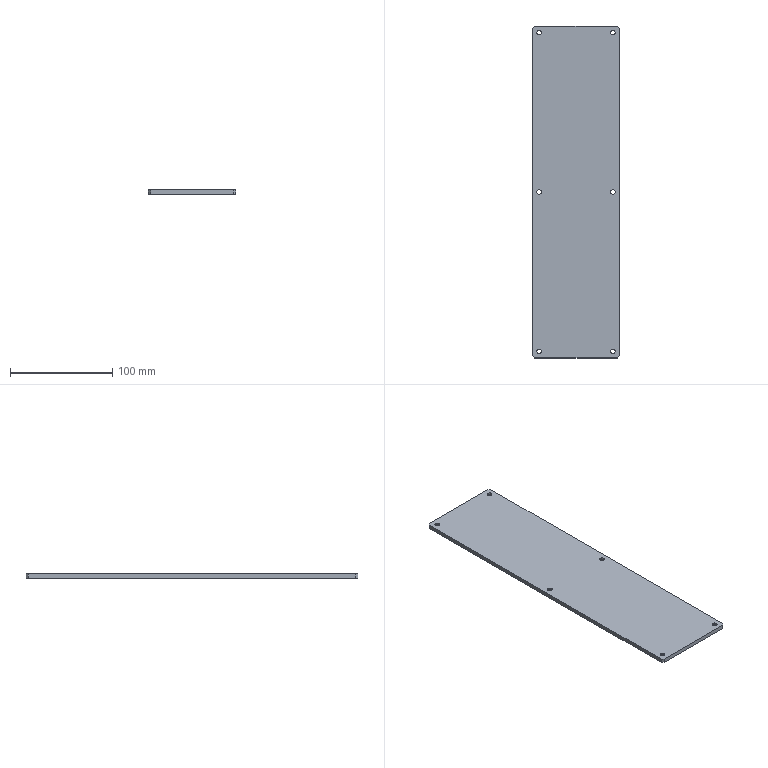Part | STEP file | 11-FG-SZ02911 | 1 solid | 34 faces | box 85 x 324 x 4 mm | volume 109466 mm3 | cone 12 | cylinder 12 | plane 10 | commonest cylinder face diameters 4.5 x12
STEP:
#1=CARTESIAN_POINT('',(-33.75,-155.5,2.23));
#2=VERTEX_POINT('',#1);
#3=CARTESIAN_POINT('',(-38.25,-155.5,2.23));
#4=VERTEX_POINT('',#3);
#5=CARTESIAN_POINT('',(-36.,-155.5,2.23));
#6=DIRECTION('',(0.,0.,-1.));
#7=DIRECTION('',(-1.,0.,0.));
#8=AXIS2_PLACEMENT_3D('',#5,#6,#7);
#9=CIRCLE('',#8,2.25);
#10=EDGE_CURVE('',#2,#4,#9,.T.);
#11=ORIENTED_EDGE('',*,*,#10,.F.);
#12=CARTESIAN_POINT('',(-31.52,-155.5,0.));
#13=VERTEX_POINT('',#12);
#14=CARTESIAN_POINT('',(-31.52,-155.5,0.));
#15=DIRECTION('',(0.7071,0.,-0.7071));
#16=VECTOR('',#15,1000.);
#17=LINE('',#14,#16);
#18=EDGE_CURVE('',#2,#13,#17,.T.);
#19=ORIENTED_EDGE('',*,*,#18,.T.);
#20=CARTESIAN_POINT('',(-40.48,-155.5,0.));
#21=VERTEX_POINT('',#20);
#22=CARTESIAN_POINT('',(-36.,-155.5,0.));
#23=DIRECTION('',(0.,0.,-1.));
#24=DIRECTION('',(-1.,0.,0.));
#25=AXIS2_PLACEMENT_3D('',#22,#23,#24);
#26=CIRCLE('',#25,4.48);
#27=EDGE_CURVE('',#13,#21,#26,.T.);
#28=ORIENTED_EDGE('',*,*,#27,.T.);
#29=CARTESIAN_POINT('',(-40.48,-155.5,0.));
#30=DIRECTION('',(-0.7071,0.,-0.7071));
#31=VECTOR('',#30,1000.);
#32=LINE('',#29,#31);
#33=EDGE_CURVE('',#4,#21,#32,.T.);
#34=ORIENTED_EDGE('',*,*,#33,.F.);
#35=EDGE_LOOP('',(#11,#19,#28,#34));
#36=FACE_OUTER_BOUND('',#35,.T.);
#37=CARTESIAN_POINT('',(-36.,-155.5,0.));
#38=DIRECTION('',(0.,0.,-1.));
#39=DIRECTION('',(-1.,0.,0.));
#40=AXIS2_PLACEMENT_3D('',#37,#38,#39);
#41=CONICAL_SURFACE('',#40,4.48,0.7854);
#42=ADVANCED_FACE('',(#36),#41,.F.);
#43=CARTESIAN_POINT('',(-38.25,-155.5,4.));
#44=VERTEX_POINT('',#43);
#45=CARTESIAN_POINT('',(-33.75,-155.5,4.));
#46=VERTEX_POINT('',#45);
#47=CARTESIAN_POINT('',(-36.,-155.5,4.));
#48=DIRECTION('',(0.,0.,1.));
#49=DIRECTION('',(1.,0.,0.));
#50=AXIS2_PLACEMENT_3D('',#47,#48,#49);
#51=CIRCLE('',#50,2.25);
#52=EDGE_CURVE('',#44,#46,#51,.T.);
#53=ORIENTED_EDGE('',*,*,#52,.T.);
#54=CARTESIAN_POINT('',(-33.75,-155.5,0.));
#55=DIRECTION('',(0.,0.,-1.));
#56=VECTOR('',#55,1000.);
#57=LINE('',#54,#56);
#58=EDGE_CURVE('',#46,#2,#57,.T.);
#59=ORIENTED_EDGE('',*,*,#58,.T.);
#60=ORIENTED_EDGE('',*,*,#10,.T.);
#61=CARTESIAN_POINT('',(-38.25,-155.5,0.));
#62=DIRECTION('',(0.,0.,-1.));
#63=VECTOR('',#62,1000.);
#64=LINE('',#61,#63);
#65=EDGE_CURVE('',#44,#4,#64,.T.);
#66=ORIENTED_EDGE('',*,*,#65,.F.);
#67=EDGE_LOOP('',(#53,#59,#60,#66));
#68=FACE_OUTER_BOUND('',#67,.T.);
#69=CARTESIAN_POINT('',(-36.,-155.5,0.));
#70=DIRECTION('',(0.,0.,-1.));
#71=DIRECTION('',(-1.,0.,0.));
#72=AXIS2_PLACEMENT_3D('',#69,#70,#71);
#73=CYLINDRICAL_SURFACE('',#72,2.25);
#74=ADVANCED_FACE('',(#68),#73,.F.);
#75=CARTESIAN_POINT('',(-33.75,155.5,2.23));
#76=VERTEX_POINT('',#75);
#77=CARTESIAN_POINT('',(-38.25,155.5,2.23));
#78=VERTEX_POINT('',#77);
#79=CARTESIAN_POINT('',(-36.,155.5,2.23));
#80=DIRECTION('',(0.,0.,-1.));
#81=DIRECTION('',(-1.,0.,0.));
#82=AXIS2_PLACEMENT_3D('',#79,#80,#81);
#83=CIRCLE('',#82,2.25);
#84=EDGE_CURVE('',#76,#78,#83,.T.);
#85=ORIENTED_EDGE('',*,*,#84,.F.);
#86=CARTESIAN_POINT('',(-31.52,155.5,0.));
#87=VERTEX_POINT('',#86);
#88=CARTESIAN_POINT('',(-31.52,155.5,0.));
#89=DIRECTION('',(0.7071,0.,-0.7071));
#90=VECTOR('',#89,1000.);
#91=LINE('',#88,#90);
#92=EDGE_CURVE('',#76,#87,#91,.T.);
#93=ORIENTED_EDGE('',*,*,#92,.T.);
#94=CARTESIAN_POINT('',(-40.48,155.5,0.));
#95=VERTEX_POINT('',#94);
#96=CARTESIAN_POINT('',(-36.,155.5,0.));
#97=DIRECTION('',(0.,0.,-1.));
#98=DIRECTION('',(-1.,0.,0.));
#99=AXIS2_PLACEMENT_3D('',#96,#97,#98);
#100=CIRCLE('',#99,4.48);
#101=EDGE_CURVE('',#87,#95,#100,.T.);
#102=ORIENTED_EDGE('',*,*,#101,.T.);
#103=CARTESIAN_POINT('',(-40.48,155.5,0.));
#104=DIRECTION('',(-0.7071,0.,-0.7071));
#105=VECTOR('',#104,1000.);
#106=LINE('',#103,#105);
#107=EDGE_CURVE('',#78,#95,#106,.T.);
#108=ORIENTED_EDGE('',*,*,#107,.F.);
#109=EDGE_LOOP('',(#85,#93,#102,#108));
#110=FACE_OUTER_BOUND('',#109,.T.);
#111=CARTESIAN_POINT('',(-36.,155.5,0.));
#112=DIRECTION('',(0.,0.,-1.));
#113=DIRECTION('',(-1.,0.,0.));
#114=AXIS2_PLACEMENT_3D('',#111,#112,#113);
#115=CONICAL_SURFACE('',#114,4.48,0.7854);
#116=ADVANCED_FACE('',(#110),#115,.F.);
#117=CARTESIAN_POINT('',(-38.25,155.5,4.));
#118=VERTEX_POINT('',#117);
#119=CARTESIAN_POINT('',(-33.75,155.5,4.));
#120=VERTEX_POINT('',#119);
#121=CARTESIAN_POINT('',(-36.,155.5,4.));
#122=DIRECTION('',(0.,0.,1.));
#123=DIRECTION('',(1.,0.,0.));
#124=AXIS2_PLACEMENT_3D('',#121,#122,#123);
#125=CIRCLE('',#124,2.25);
#126=EDGE_CURVE('',#118,#120,#125,.T.);
#127=ORIENTED_EDGE('',*,*,#126,.T.);
#128=CARTESIAN_POINT('',(-33.75,155.5,0.));
#129=DIRECTION('',(0.,0.,-1.));
#130=VECTOR('',#129,1000.);
#131=LINE('',#128,#130);
#132=EDGE_CURVE('',#120,#76,#131,.T.);
#133=ORIENTED_EDGE('',*,*,#132,.T.);
#134=ORIENTED_EDGE('',*,*,#84,.T.);
#135=CARTESIAN_POINT('',(-38.25,155.5,0.));
#136=DIRECTION('',(0.,0.,-1.));
#137=VECTOR('',#136,1000.);
#138=LINE('',#135,#137);
#139=EDGE_CURVE('',#118,#78,#138,.T.);
#140=ORIENTED_EDGE('',*,*,#139,.F.);
#141=EDGE_LOOP('',(#127,#133,#134,#140));
#142=FACE_OUTER_BOUND('',#141,.T.);
#143=CARTESIAN_POINT('',(-36.,155.5,0.));
#144=DIRECTION('',(0.,0.,-1.));
#145=DIRECTION('',(-1.,0.,0.));
#146=AXIS2_PLACEMENT_3D('',#143,#144,#145);
#147=CYLINDRICAL_SURFACE('',#146,2.25);
#148=ADVANCED_FACE('',(#142),#147,.F.);
#149=CARTESIAN_POINT('',(-33.75,0.,2.23));
#150=VERTEX_POINT('',#149);
#151=CARTESIAN_POINT('',(-38.25,0.,2.23));
#152=VERTEX_POINT('',#151);
#153=CARTESIAN_POINT('',(-36.,0.,2.23));
#154=DIRECTION('',(0.,0.,-1.));
#155=DIRECTION('',(-1.,0.,0.));
#156=AXIS2_PLACEMENT_3D('',#153,#154,#155);
#157=CIRCLE('',#156,2.25);
#158=EDGE_CURVE('',#150,#152,#157,.T.);
#159=ORIENTED_EDGE('',*,*,#158,.F.);
#160=CARTESIAN_POINT('',(-31.52,0.,0.));
#161=VERTEX_POINT('',#160);
#162=CARTESIAN_POINT('',(-31.52,0.,0.));
#163=DIRECTION('',(0.7071,0.,-0.7071));
#164=VECTOR('',#163,1000.);
#165=LINE('',#162,#164);
#166=EDGE_CURVE('',#150,#161,#165,.T.);
#167=ORIENTED_EDGE('',*,*,#166,.T.);
#168=CARTESIAN_POINT('',(-40.48,0.,0.));
#169=VERTEX_POINT('',#168);
#170=CARTESIAN_POINT('',(-36.,0.,0.));
#171=DIRECTION('',(0.,0.,-1.));
#172=DIRECTION('',(-1.,0.,0.));
#173=AXIS2_PLACEMENT_3D('',#170,#171,#172);
#174=CIRCLE('',#173,4.48);
#175=EDGE_CURVE('',#161,#169,#174,.T.);
#176=ORIENTED_EDGE('',*,*,#175,.T.);
#177=CARTESIAN_POINT('',(-40.48,0.,0.));
#178=DIRECTION('',(-0.7071,0.,-0.7071));
#179=VECTOR('',#178,1000.);
#180=LINE('',#177,#179);
#181=EDGE_CURVE('',#152,#169,#180,.T.);
#182=ORIENTED_EDGE('',*,*,#181,.F.);
#183=EDGE_LOOP('',(#159,#167,#176,#182));
#184=FACE_OUTER_BOUND('',#183,.T.);
#185=CARTESIAN_POINT('',(-36.,0.,0.));
#186=DIRECTION('',(0.,0.,-1.));
#187=DIRECTION('',(-1.,0.,0.));
#188=AXIS2_PLACEMENT_3D('',#185,#186,#187);
#189=CONICAL_SURFACE('',#188,4.48,0.7854);
#190=ADVANCED_FACE('',(#184),#189,.F.);
#191=CARTESIAN_POINT('',(-38.25,0.,4.));
#192=VERTEX_POINT('',#191);
#193=CARTESIAN_POINT('',(-33.75,0.,4.));
#194=VERTEX_POINT('',#193);
#195=CARTESIAN_POINT('',(-36.,0.,4.));
#196=DIRECTION('',(0.,0.,1.));
#197=DIRECTION('',(1.,0.,0.));
#198=AXIS2_PLACEMENT_3D('',#195,#196,#197);
#199=CIRCLE('',#198,2.25);
#200=EDGE_CURVE('',#192,#194,#199,.T.);
#201=ORIENTED_EDGE('',*,*,#200,.T.);
#202=CARTESIAN_POINT('',(-33.75,0.,0.));
#203=DIRECTION('',(0.,0.,-1.));
#204=VECTOR('',#203,1000.);
#205=LINE('',#202,#204);
#206=EDGE_CURVE('',#194,#150,#205,.T.);
#207=ORIENTED_EDGE('',*,*,#206,.T.);
#208=ORIENTED_EDGE('',*,*,#158,.T.);
#209=CARTESIAN_POINT('',(-38.25,0.,0.));
#210=DIRECTION('',(0.,0.,-1.));
#211=VECTOR('',#210,1000.);
#212=LINE('',#209,#211);
#213=EDGE_CURVE('',#192,#152,#212,.T.);
#214=ORIENTED_EDGE('',*,*,#213,.F.);
#215=EDGE_LOOP('',(#201,#207,#208,#214));
#216=FACE_OUTER_BOUND('',#215,.T.);
#217=CARTESIAN_POINT('',(-36.,0.,0.));
#218=DIRECTION('',(0.,0.,-1.));
#219=DIRECTION('',(-1.,0.,0.));
#220=AXIS2_PLACEMENT_3D('',#217,#218,#219);
#221=CYLINDRICAL_SURFACE('',#220,2.25);
#222=ADVANCED_FACE('',(#216),#221,.F.);
#223=CARTESIAN_POINT('',(38.25,-155.5,2.23));
#224=VERTEX_POINT('',#223);
#225=CARTESIAN_POINT('',(33.75,-155.5,2.23));
#226=VERTEX_POINT('',#225);
#227=CARTESIAN_POINT('',(36.,-155.5,2.23));
#228=DIRECTION('',(0.,0.,-1.));
#229=DIRECTION('',(-1.,0.,0.));
#230=AXIS2_PLACEMENT_3D('',#227,#228,#229);
#231=CIRCLE('',#230,2.25);
#232=EDGE_CURVE('',#224,#226,#231,.T.);
#233=ORIENTED_EDGE('',*,*,#232,.F.);
#234=CARTESIAN_POINT('',(40.48,-155.5,0.));
#235=VERTEX_POINT('',#234);
#236=CARTESIAN_POINT('',(40.48,-155.5,0.));
#237=DIRECTION('',(0.7071,0.,-0.7071));
#238=VECTOR('',#237,1000.);
#239=LINE('',#236,#238);
#240=EDGE_CURVE('',#224,#235,#239,.T.);
#241=ORIENTED_EDGE('',*,*,#240,.T.);
#242=CARTESIAN_POINT('',(31.52,-155.5,0.));
#243=VERTEX_POINT('',#242);
#244=CARTESIAN_POINT('',(36.,-155.5,0.));
#245=DIRECTION('',(0.,0.,-1.));
#246=DIRECTION('',(-1.,0.,0.));
#247=AXIS2_PLACEMENT_3D('',#244,#245,#246);
#248=CIRCLE('',#247,4.48);
#249=EDGE_CURVE('',#235,#243,#248,.T.);
#250=ORIENTED_EDGE('',*,*,#249,.T.);
#251=CARTESIAN_POINT('',(31.52,-155.5,0.));
#252=DIRECTION('',(-0.7071,0.,-0.7071));
#253=VECTOR('',#252,1000.);
#254=LINE('',#251,#253);
#255=EDGE_CURVE('',#226,#243,#254,.T.);
#256=ORIENTED_EDGE('',*,*,#255,.F.);
#257=EDGE_LOOP('',(#233,#241,#250,#256));
#258=FACE_OUTER_BOUND('',#257,.T.);
#259=CARTESIAN_POINT('',(36.,-155.5,0.));
#260=DIRECTION('',(0.,0.,-1.));
#261=DIRECTION('',(-1.,0.,0.));
#262=AXIS2_PLACEMENT_3D('',#259,#260,#261);
#263=CONICAL_SURFACE('',#262,4.48,0.7854);
#264=ADVANCED_FACE('',(#258),#263,.F.);
#265=CARTESIAN_POINT('',(33.75,-155.5,4.));
#266=VERTEX_POINT('',#265);
#267=CARTESIAN_POINT('',(38.25,-155.5,4.));
#268=VERTEX_POINT('',#267);
#269=CARTESIAN_POINT('',(36.,-155.5,4.));
#270=DIRECTION('',(0.,0.,1.));
#271=DIRECTION('',(1.,0.,0.));
#272=AXIS2_PLACEMENT_3D('',#269,#270,#271);
#273=CIRCLE('',#272,2.25);
#274=EDGE_CURVE('',#266,#268,#273,.T.);
#275=ORIENTED_EDGE('',*,*,#274,.T.);
#276=CARTESIAN_POINT('',(38.25,-155.5,0.));
#277=DIRECTION('',(0.,0.,-1.));
#278=VECTOR('',#277,1000.);
#279=LINE('',#276,#278);
#280=EDGE_CURVE('',#268,#224,#279,.T.);
#281=ORIENTED_EDGE('',*,*,#280,.T.);
#282=ORIENTED_EDGE('',*,*,#232,.T.);
#283=CARTESIAN_POINT('',(33.75,-155.5,0.));
#284=DIRECTION('',(0.,0.,-1.));
#285=VECTOR('',#284,1000.);
#286=LINE('',#283,#285);
#287=EDGE_CURVE('',#266,#226,#286,.T.);
#288=ORIENTED_EDGE('',*,*,#287,.F.);
#289=EDGE_LOOP('',(#275,#281,#282,#288));
#290=FACE_OUTER_BOUND('',#289,.T.);
#291=CARTESIAN_POINT('',(36.,-155.5,0.));
#292=DIRECTION('',(0.,0.,-1.));
#293=DIRECTION('',(-1.,0.,0.));
#294=AXIS2_PLACEMENT_3D('',#291,#292,#293);
#295=CYLINDRICAL_SURFACE('',#294,2.25);
#296=ADVANCED_FACE('',(#290),#295,.F.);
#297=CARTESIAN_POINT('',(38.25,155.5,2.23));
#298=VERTEX_POINT('',#297);
#299=CARTESIAN_POINT('',(33.75,155.5,2.23));
#300=VERTEX_POINT('',#299);
#301=CARTESIAN_POINT('',(36.,155.5,2.23));
#302=DIRECTION('',(0.,0.,-1.));
#303=DIRECTION('',(-1.,0.,0.));
#304=AXIS2_PLACEMENT_3D('',#301,#302,#303);
#305=CIRCLE('',#304,2.25);
#306=EDGE_CURVE('',#298,#300,#305,.T.);
#307=ORIENTED_EDGE('',*,*,#306,.F.);
#308=CARTESIAN_POINT('',(40.48,155.5,0.));
#309=VERTEX_POINT('',#308);
#310=CARTESIAN_POINT('',(40.48,155.5,0.));
#311=DIRECTION('',(0.7071,0.,-0.7071));
#312=VECTOR('',#311,1000.);
#313=LINE('',#310,#312);
#314=EDGE_CURVE('',#298,#309,#313,.T.);
#315=ORIENTED_EDGE('',*,*,#314,.T.);
#316=CARTESIAN_POINT('',(31.52,155.5,0.));
#317=VERTEX_POINT('',#316);
#318=CARTESIAN_POINT('',(36.,155.5,0.));
#319=DIRECTION('',(0.,0.,-1.));
#320=DIRECTION('',(-1.,0.,0.));
#321=AXIS2_PLACEMENT_3D('',#318,#319,#320);
#322=CIRCLE('',#321,4.48);
#323=EDGE_CURVE('',#309,#317,#322,.T.);
#324=ORIENTED_EDGE('',*,*,#323,.T.);
#325=CARTESIAN_POINT('',(31.52,155.5,0.));
#326=DIRECTION('',(-0.7071,0.,-0.7071));
#327=VECTOR('',#326,1000.);
#328=LINE('',#325,#327);
#329=EDGE_CURVE('',#300,#317,#328,.T.);
#330=ORIENTED_EDGE('',*,*,#329,.F.);
#331=EDGE_LOOP('',(#307,#315,#324,#330));
#332=FACE_OUTER_BOUND('',#331,.T.);
#333=CARTESIAN_POINT('',(36.,155.5,0.));
#334=DIRECTION('',(0.,0.,-1.));
#335=DIRECTION('',(-1.,0.,0.));
#336=AXIS2_PLACEMENT_3D('',#333,#334,#335);
#337=CONICAL_SURFACE('',#336,4.48,0.7854);
#338=ADVANCED_FACE('',(#332),#337,.F.);
#339=CARTESIAN_POINT('',(33.75,155.5,4.));
#340=VERTEX_POINT('',#339);
#341=CARTESIAN_POINT('',(38.25,155.5,4.));
#342=VERTEX_POINT('',#341);
#343=CARTESIAN_POINT('',(36.,155.5,4.));
#344=DIRECTION('',(0.,0.,1.));
#345=DIRECTION('',(1.,0.,0.));
#346=AXIS2_PLACEMENT_3D('',#343,#344,#345);
#347=CIRCLE('',#346,2.25);
#348=EDGE_CURVE('',#340,#342,#347,.T.);
#349=ORIENTED_EDGE('',*,*,#348,.T.);
#350=CARTESIAN_POINT('',(38.25,155.5,0.));
#351=DIRECTION('',(0.,0.,-1.));
#352=VECTOR('',#351,1000.);
#353=LINE('',#350,#352);
#354=EDGE_CURVE('',#342,#298,#353,.T.);
#355=ORIENTED_EDGE('',*,*,#354,.T.);
#356=ORIENTED_EDGE('',*,*,#306,.T.);
#357=CARTESIAN_POINT('',(33.75,155.5,0.));
#358=DIRECTION('',(0.,0.,-1.));
#359=VECTOR('',#358,1000.);
#360=LINE('',#357,#359);
#361=EDGE_CURVE('',#340,#300,#360,.T.);
#362=ORIENTED_EDGE('',*,*,#361,.F.);
#363=EDGE_LOOP('',(#349,#355,#356,#362));
#364=FACE_OUTER_BOUND('',#363,.T.);
#365=CARTESIAN_POINT('',(36.,155.5,0.));
#366=DIRECTION('',(0.,0.,-1.));
#367=DIRECTION('',(-1.,0.,0.));
#368=AXIS2_PLACEMENT_3D('',#365,#366,#367);
#369=CYLINDRICAL_SURFACE('',#368,2.25);
#370=ADVANCED_FACE('',(#364),#369,.F.);
#371=CARTESIAN_POINT('',(38.25,0.,2.23));
#372=VERTEX_POINT('',#371);
#373=CARTESIAN_POINT('',(33.75,0.,2.23));
#374=VERTEX_POINT('',#373);
#375=CARTESIAN_POINT('',(36.,0.,2.23));
#376=DIRECTION('',(0.,0.,-1.));
#377=DIRECTION('',(-1.,0.,0.));
#378=AXIS2_PLACEMENT_3D('',#375,#376,#377);
#379=CIRCLE('',#378,2.25);
#380=EDGE_CURVE('',#372,#374,#379,.T.);
#381=ORIENTED_EDGE('',*,*,#380,.F.);
#382=CARTESIAN_POINT('',(40.48,0.,0.));
#383=VERTEX_POINT('',#382);
#384=CARTESIAN_POINT('',(40.48,0.,0.));
#385=DIRECTION('',(0.7071,0.,-0.7071));
#386=VECTOR('',#385,1000.);
#387=LINE('',#384,#386);
#388=EDGE_CURVE('',#372,#383,#387,.T.);
#389=ORIENTED_EDGE('',*,*,#388,.T.);
#390=CARTESIAN_POINT('',(31.52,0.,0.));
#391=VERTEX_POINT('',#390);
#392=CARTESIAN_POINT('',(36.,0.,0.));
#393=DIRECTION('',(0.,0.,-1.));
#394=DIRECTION('',(-1.,0.,0.));
#395=AXIS2_PLACEMENT_3D('',#392,#393,#394);
#396=CIRCLE('',#395,4.48);
#397=EDGE_CURVE('',#383,#391,#396,.T.);
#398=ORIENTED_EDGE('',*,*,#397,.T.);
#399=CARTESIAN_POINT('',(31.52,0.,0.));
#400=DIRECTION('',(-0.7071,0.,-0.7071));
#401=VECTOR('',#400,1000.);
#402=LINE('',#399,#401);
#403=EDGE_CURVE('',#374,#391,#402,.T.);
#404=ORIENTED_EDGE('',*,*,#403,.F.);
#405=EDGE_LOOP('',(#381,#389,#398,#404));
#406=FACE_OUTER_BOUND('',#405,.T.);
#407=CARTESIAN_POINT('',(36.,0.,0.));
#408=DIRECTION('',(0.,0.,-1.));
#409=DIRECTION('',(-1.,0.,0.));
#410=AXIS2_PLACEMENT_3D('',#407,#408,#409);
#411=CONICAL_SURFACE('',#410,4.48,0.7854);
#412=ADVANCED_FACE('',(#406),#411,.F.);
#413=CARTESIAN_POINT('',(33.75,0.,4.));
#414=VERTEX_POINT('',#413);
#415=CARTESIAN_POINT('',(38.25,0.,4.));
#416=VERTEX_POINT('',#415);
#417=CARTESIAN_POINT('',(36.,0.,4.));
#418=DIRECTION('',(0.,0.,1.));
#419=DIRECTION('',(1.,0.,0.));
#420=AXIS2_PLACEMENT_3D('',#417,#418,#419);
#421=CIRCLE('',#420,2.25);
#422=EDGE_CURVE('',#414,#416,#421,.T.);
#423=ORIENTED_EDGE('',*,*,#422,.T.);
#424=CARTESIAN_POINT('',(38.25,0.,0.));
#425=DIRECTION('',(0.,0.,-1.));
#426=VECTOR('',#425,1000.);
#427=LINE('',#424,#426);
#428=EDGE_CURVE('',#416,#372,#427,.T.);
#429=ORIENTED_EDGE('',*,*,#428,.T.);
#430=ORIENTED_EDGE('',*,*,#380,.T.);
#431=CARTESIAN_POINT('',(33.75,0.,0.));
#432=DIRECTION('',(0.,0.,-1.));
#433=VECTOR('',#432,1000.);
#434=LINE('',#431,#433);
#435=EDGE_CURVE('',#414,#374,#434,.T.);
#436=ORIENTED_EDGE('',*,*,#435,.F.);
#437=EDGE_LOOP('',(#423,#429,#430,#436));
#438=FACE_OUTER_BOUND('',#437,.T.);
#439=CARTESIAN_POINT('',(36.,0.,0.));
#440=DIRECTION('',(0.,0.,-1.));
#441=DIRECTION('',(-1.,0.,0.));
#442=AXIS2_PLACEMENT_3D('',#439,#440,#441);
#443=CYLINDRICAL_SURFACE('',#442,2.25);
#444=ADVANCED_FACE('',(#438),#443,.F.);
#445=CARTESIAN_POINT('',(-42.5,160.,0.));
#446=VERTEX_POINT('',#445);
#447=CARTESIAN_POINT('',(-42.5,-160.,0.));
#448=VERTEX_POINT('',#447);
#449=CARTESIAN_POINT('',(-42.5,-162.,0.));
#450=DIRECTION('',(0.,-1.,0.));
#451=VECTOR('',#450,1000.);
#452=LINE('',#449,#451);
#453=EDGE_CURVE('',#446,#448,#452,.T.);
#454=ORIENTED_EDGE('',*,*,#453,.T.);
#455=CARTESIAN_POINT('',(-42.5,-160.,4.));
#456=VERTEX_POINT('',#455);
#457=CARTESIAN_POINT('',(-42.5,-160.,4.));
#458=DIRECTION('',(0.,0.,1.));
#459=VECTOR('',#458,1000.);
#460=LINE('',#457,#459);
#461=EDGE_CURVE('',#448,#456,#460,.T.);
#462=ORIENTED_EDGE('',*,*,#461,.T.);
#463=CARTESIAN_POINT('',(-42.5,160.,4.));
#464=VERTEX_POINT('',#463);
#465=CARTESIAN_POINT('',(-42.5,-162.,4.));
#466=DIRECTION('',(0.,-1.,0.));
#467=VECTOR('',#466,1000.);
#468=LINE('',#465,#467);
#469=EDGE_CURVE('',#464,#456,#468,.T.);
#470=ORIENTED_EDGE('',*,*,#469,.F.);
#471=CARTESIAN_POINT('',(-42.5,160.,4.));
#472=DIRECTION('',(0.,0.,-1.));
#473=VECTOR('',#472,1000.);
#474=LINE('',#471,#473);
#475=EDGE_CURVE('',#464,#446,#474,.T.);
#476=ORIENTED_EDGE('',*,*,#475,.T.);
#477=EDGE_LOOP('',(#454,#462,#470,#476));
#478=FACE_OUTER_BOUND('',#477,.T.);
#479=CARTESIAN_POINT('',(-42.5,-162.,4.));
#480=DIRECTION('',(1.,0.,0.));
#481=DIRECTION('',(0.,0.,-1.));
#482=AXIS2_PLACEMENT_3D('',#479,#480,#481);
#483=PLANE('',#482);
#484=ADVANCED_FACE('',(#478),#483,.F.);
#485=CARTESIAN_POINT('',(-40.5,-162.,4.));
#486=VERTEX_POINT('',#485);
#487=CARTESIAN_POINT('',(40.5,-162.,4.));
#488=VERTEX_POINT('',#487);
#489=CARTESIAN_POINT('',(42.5,-162.,4.));
#490=DIRECTION('',(1.,0.,0.));
#491=VECTOR('',#490,1000.);
#492=LINE('',#489,#491);
#493=EDGE_CURVE('',#486,#488,#492,.T.);
#494=ORIENTED_EDGE('',*,*,#493,.F.);
#495=CARTESIAN_POINT('',(-40.5,-162.,0.));
#496=VERTEX_POINT('',#495);
#497=CARTESIAN_POINT('',(-40.5,-162.,4.));
#498=DIRECTION('',(0.,0.,-1.));
#499=VECTOR('',#498,1000.);
#500=LINE('',#497,#499);
#501=EDGE_CURVE('',#486,#496,#500,.T.);
#502=ORIENTED_EDGE('',*,*,#501,.T.);
#503=CARTESIAN_POINT('',(40.5,-162.,0.));
#504=VERTEX_POINT('',#503);
#505=CARTESIAN_POINT('',(42.5,-162.,0.));
#506=DIRECTION('',(1.,0.,0.));
#507=VECTOR('',#506,1000.);
#508=LINE('',#505,#507);
#509=EDGE_CURVE('',#496,#504,#508,.T.);
#510=ORIENTED_EDGE('',*,*,#509,.T.);
#511=CARTESIAN_POINT('',(40.5,-162.,4.));
#512=DIRECTION('',(0.,0.,1.));
#513=VECTOR('',#512,1000.);
#514=LINE('',#511,#513);
#515=EDGE_CURVE('',#504,#488,#514,.T.);
#516=ORIENTED_EDGE('',*,*,#515,.T.);
#517=EDGE_LOOP('',(#494,#502,#510,#516));
#518=FACE_OUTER_BOUND('',#517,.T.);
#519=CARTESIAN_POINT('',(42.5,-162.,4.));
#520=DIRECTION('',(0.,1.,0.));
#521=DIRECTION('',(0.,0.,1.));
#522=AXIS2_PLACEMENT_3D('',#519,#520,#521);
#523=PLANE('',#522);
#524=ADVANCED_FACE('',(#518),#523,.F.);
#525=CARTESIAN_POINT('',(42.5,-160.,4.));
#526=VERTEX_POINT('',#525);
#527=CARTESIAN_POINT('',(42.5,160.,4.));
#528=VERTEX_POINT('',#527);
#529=CARTESIAN_POINT('',(42.5,-162.,4.));
#530=DIRECTION('',(0.,1.,0.));
#531=VECTOR('',#530,1000.);
#532=LINE('',#529,#531);
#533=EDGE_CURVE('',#526,#528,#532,.T.);
#534=ORIENTED_EDGE('',*,*,#533,.F.);
#535=CARTESIAN_POINT('',(42.5,-160.,0.));
#536=VERTEX_POINT('',#535);
#537=CARTESIAN_POINT('',(42.5,-160.,4.));
#538=DIRECTION('',(0.,0.,-1.));
#539=VECTOR('',#538,1000.);
#540=LINE('',#537,#539);
#541=EDGE_CURVE('',#526,#536,#540,.T.);
#542=ORIENTED_EDGE('',*,*,#541,.T.);
#543=CARTESIAN_POINT('',(42.5,160.,0.));
#544=VERTEX_POINT('',#543);
#545=CARTESIAN_POINT('',(42.5,-162.,0.));
#546=DIRECTION('',(0.,1.,0.));
#547=VECTOR('',#546,1000.);
#548=LINE('',#545,#547);
#549=EDGE_CURVE('',#536,#544,#548,.T.);
#550=ORIENTED_EDGE('',*,*,#549,.T.);
#551=CARTESIAN_POINT('',(42.5,160.,4.));
#552=DIRECTION('',(0.,0.,1.));
#553=VECTOR('',#552,1000.);
#554=LINE('',#551,#553);
#555=EDGE_CURVE('',#544,#528,#554,.T.);
#556=ORIENTED_EDGE('',*,*,#555,.T.);
#557=EDGE_LOOP('',(#534,#542,#550,#556));
#558=FACE_OUTER_BOUND('',#557,.T.);
#559=CARTESIAN_POINT('',(42.5,-162.,4.));
#560=DIRECTION('',(-1.,0.,0.));
#561=DIRECTION('',(0.,0.,1.));
#562=AXIS2_PLACEMENT_3D('',#559,#560,#561);
#563=PLANE('',#562);
#564=ADVANCED_FACE('',(#558),#563,.F.);
#565=CARTESIAN_POINT('',(40.5,162.,4.));
#566=VERTEX_POINT('',#565);
#567=CARTESIAN_POINT('',(-40.5,162.,4.));
#568=VERTEX_POINT('',#567);
#569=CARTESIAN_POINT('',(42.5,162.,4.));
#570=DIRECTION('',(-1.,0.,0.));
#571=VECTOR('',#570,1000.);
#572=LINE('',#569,#571);
#573=EDGE_CURVE('',#566,#568,#572,.T.);
#574=ORIENTED_EDGE('',*,*,#573,.F.);
#575=CARTESIAN_POINT('',(40.5,162.,0.));
#576=VERTEX_POINT('',#575);
#577=CARTESIAN_POINT('',(40.5,162.,4.));
#578=DIRECTION('',(0.,0.,-1.));
#579=VECTOR('',#578,1000.);
#580=LINE('',#577,#579);
#581=EDGE_CURVE('',#566,#576,#580,.T.);
#582=ORIENTED_EDGE('',*,*,#581,.T.);
#583=CARTESIAN_POINT('',(-40.5,162.,0.));
#584=VERTEX_POINT('',#583);
#585=CARTESIAN_POINT('',(42.5,162.,0.));
#586=DIRECTION('',(-1.,0.,0.));
#587=VECTOR('',#586,1000.);
#588=LINE('',#585,#587);
#589=EDGE_CURVE('',#576,#584,#588,.T.);
#590=ORIENTED_EDGE('',*,*,#589,.T.);
#591=CARTESIAN_POINT('',(-40.5,162.,4.));
#592=DIRECTION('',(0.,0.,1.));
#593=VECTOR('',#592,1000.);
#594=LINE('',#591,#593);
#595=EDGE_CURVE('',#584,#568,#594,.T.);
#596=ORIENTED_EDGE('',*,*,#595,.T.);
#597=EDGE_LOOP('',(#574,#582,#590,#596));
#598=FACE_OUTER_BOUND('',#597,.T.);
#599=CARTESIAN_POINT('',(42.5,162.,4.));
#600=DIRECTION('',(0.,-1.,0.));
#601=DIRECTION('',(0.,0.,-1.));
#602=AXIS2_PLACEMENT_3D('',#599,#600,#601);
#603=PLANE('',#602);
#604=ADVANCED_FACE('',(#598),#603,.F.);
#605=ORIENTED_EDGE('',*,*,#52,.F.);
#606=CARTESIAN_POINT('',(-36.,-155.5,4.));
#607=DIRECTION('',(0.,0.,1.));
#608=DIRECTION('',(1.,0.,0.));
#609=AXIS2_PLACEMENT_3D('',#606,#607,#608);
#610=CIRCLE('',#609,2.25);
#611=EDGE_CURVE('',#46,#44,#610,.T.);
#612=ORIENTED_EDGE('',*,*,#611,.F.);
#613=EDGE_LOOP('',(#605,#612));
#614=FACE_BOUND('',#613,.T.);
#615=ORIENTED_EDGE('',*,*,#126,.F.);
#616=CARTESIAN_POINT('',(-36.,155.5,4.));
#617=DIRECTION('',(0.,0.,1.));
#618=DIRECTION('',(1.,0.,0.));
#619=AXIS2_PLACEMENT_3D('',#616,#617,#618);
#620=CIRCLE('',#619,2.25);
#621=EDGE_CURVE('',#120,#118,#620,.T.);
#622=ORIENTED_EDGE('',*,*,#621,.F.);
#623=EDGE_LOOP('',(#615,#622));
#624=FACE_BOUND('',#623,.T.);
#625=ORIENTED_EDGE('',*,*,#200,.F.);
#626=CARTESIAN_POINT('',(-36.,0.,4.));
#627=DIRECTION('',(0.,0.,1.));
#628=DIRECTION('',(1.,0.,0.));
#629=AXIS2_PLACEMENT_3D('',#626,#627,#628);
#630=CIRCLE('',#629,2.25);
#631=EDGE_CURVE('',#194,#192,#630,.T.);
#632=ORIENTED_EDGE('',*,*,#631,.F.);
#633=EDGE_LOOP('',(#625,#632));
#634=FACE_BOUND('',#633,.T.);
#635=ORIENTED_EDGE('',*,*,#274,.F.);
#636=CARTESIAN_POINT('',(36.,-155.5,4.));
#637=DIRECTION('',(0.,0.,1.));
#638=DIRECTION('',(1.,0.,0.));
#639=AXIS2_PLACEMENT_3D('',#636,#637,#638);
#640=CIRCLE('',#639,2.25);
#641=EDGE_CURVE('',#268,#266,#640,.T.);
#642=ORIENTED_EDGE('',*,*,#641,.F.);
#643=EDGE_LOOP('',(#635,#642));
#644=FACE_BOUND('',#643,.T.);
#645=ORIENTED_EDGE('',*,*,#348,.F.);
#646=CARTESIAN_POINT('',(36.,155.5,4.));
#647=DIRECTION('',(0.,0.,1.));
#648=DIRECTION('',(1.,0.,0.));
#649=AXIS2_PLACEMENT_3D('',#646,#647,#648);
#650=CIRCLE('',#649,2.25);
#651=EDGE_CURVE('',#342,#340,#650,.T.);
#652=ORIENTED_EDGE('',*,*,#651,.F.);
#653=EDGE_LOOP('',(#645,#652));
#654=FACE_BOUND('',#653,.T.);
#655=ORIENTED_EDGE('',*,*,#422,.F.);
#656=CARTESIAN_POINT('',(36.,0.,4.));
#657=DIRECTION('',(0.,0.,1.));
#658=DIRECTION('',(1.,0.,0.));
#659=AXIS2_PLACEMENT_3D('',#656,#657,#658);
#660=CIRCLE('',#659,2.25);
#661=EDGE_CURVE('',#416,#414,#660,.T.);
#662=ORIENTED_EDGE('',*,*,#661,.F.);
#663=EDGE_LOOP('',(#655,#662));
#664=FACE_BOUND('',#663,.T.);
#665=ORIENTED_EDGE('',*,*,#469,.T.);
#666=CARTESIAN_POINT('',(-101.25,-101.25,4.));
#667=DIRECTION('',(0.7071,-0.7071,0.));
#668=VECTOR('',#667,1000.);
#669=LINE('',#666,#668);
#670=EDGE_CURVE('',#456,#486,#669,.T.);
#671=ORIENTED_EDGE('',*,*,#670,.T.);
#672=ORIENTED_EDGE('',*,*,#493,.T.);
#673=CARTESIAN_POINT('',(101.25,-101.25,4.));
#674=DIRECTION('',(0.7071,0.7071,0.));
#675=VECTOR('',#674,1000.);
#676=LINE('',#673,#675);
#677=EDGE_CURVE('',#488,#526,#676,.T.);
#678=ORIENTED_EDGE('',*,*,#677,.T.);
#679=ORIENTED_EDGE('',*,*,#533,.T.);
#680=CARTESIAN_POINT('',(101.25,101.25,4.));
#681=DIRECTION('',(-0.7071,0.7071,0.));
#682=VECTOR('',#681,1000.);
#683=LINE('',#680,#682);
#684=EDGE_CURVE('',#528,#566,#683,.T.);
#685=ORIENTED_EDGE('',*,*,#684,.T.);
#686=ORIENTED_EDGE('',*,*,#573,.T.);
#687=CARTESIAN_POINT('',(-101.25,101.25,4.));
#688=DIRECTION('',(-0.7071,-0.7071,0.));
#689=VECTOR('',#688,1000.);
#690=LINE('',#687,#689);
#691=EDGE_CURVE('',#568,#464,#690,.T.);
#692=ORIENTED_EDGE('',*,*,#691,.T.);
#693=EDGE_LOOP('',(#665,#671,#672,#678,#679,#685,#686,#692));
#694=FACE_OUTER_BOUND('',#693,.T.);
#695=CARTESIAN_POINT('',(0.,0.,4.));
#696=DIRECTION('',(0.,0.,1.));
#697=DIRECTION('',(1.,0.,0.));
#698=AXIS2_PLACEMENT_3D('',#695,#696,#697);
#699=PLANE('',#698);
#700=ADVANCED_FACE('',(#614,#624,#634,#644,#654,#664,#694),#699,.T.);
#701=CARTESIAN_POINT('',(-36.,-155.5,0.));
#702=DIRECTION('',(0.,0.,-1.));
#703=DIRECTION('',(-1.,0.,0.));
#704=AXIS2_PLACEMENT_3D('',#701,#702,#703);
#705=CIRCLE('',#704,4.48);
#706=EDGE_CURVE('',#21,#13,#705,.T.);
#707=ORIENTED_EDGE('',*,*,#706,.F.);
#708=ORIENTED_EDGE('',*,*,#27,.F.);
#709=EDGE_LOOP('',(#707,#708));
#710=FACE_BOUND('',#709,.T.);
#711=CARTESIAN_POINT('',(-36.,155.5,0.));
#712=DIRECTION('',(0.,0.,-1.));
#713=DIRECTION('',(-1.,0.,0.));
#714=AXIS2_PLACEMENT_3D('',#711,#712,#713);
#715=CIRCLE('',#714,4.48);
#716=EDGE_CURVE('',#95,#87,#715,.T.);
#717=ORIENTED_EDGE('',*,*,#716,.F.);
#718=ORIENTED_EDGE('',*,*,#101,.F.);
#719=EDGE_LOOP('',(#717,#718));
#720=FACE_BOUND('',#719,.T.);
#721=CARTESIAN_POINT('',(-36.,0.,0.));
#722=DIRECTION('',(0.,0.,-1.));
#723=DIRECTION('',(-1.,0.,0.));
#724=AXIS2_PLACEMENT_3D('',#721,#722,#723);
#725=CIRCLE('',#724,4.48);
#726=EDGE_CURVE('',#169,#161,#725,.T.);
#727=ORIENTED_EDGE('',*,*,#726,.F.);
#728=ORIENTED_EDGE('',*,*,#175,.F.);
#729=EDGE_LOOP('',(#727,#728));
#730=FACE_BOUND('',#729,.T.);
#731=CARTESIAN_POINT('',(36.,-155.5,0.));
#732=DIRECTION('',(0.,0.,-1.));
#733=DIRECTION('',(-1.,0.,0.));
#734=AXIS2_PLACEMENT_3D('',#731,#732,#733);
#735=CIRCLE('',#734,4.48);
#736=EDGE_CURVE('',#243,#235,#735,.T.);
#737=ORIENTED_EDGE('',*,*,#736,.F.);
#738=ORIENTED_EDGE('',*,*,#249,.F.);
#739=EDGE_LOOP('',(#737,#738));
#740=FACE_BOUND('',#739,.T.);
#741=CARTESIAN_POINT('',(36.,155.5,0.));
#742=DIRECTION('',(0.,0.,-1.));
#743=DIRECTION('',(-1.,0.,0.));
#744=AXIS2_PLACEMENT_3D('',#741,#742,#743);
#745=CIRCLE('',#744,4.48);
#746=EDGE_CURVE('',#317,#309,#745,.T.);
#747=ORIENTED_EDGE('',*,*,#746,.F.);
#748=ORIENTED_EDGE('',*,*,#323,.F.);
#749=EDGE_LOOP('',(#747,#748));
#750=FACE_BOUND('',#749,.T.);
#751=CARTESIAN_POINT('',(36.,0.,0.));
#752=DIRECTION('',(0.,0.,-1.));
#753=DIRECTION('',(-1.,0.,0.));
#754=AXIS2_PLACEMENT_3D('',#751,#752,#753);
#755=CIRCLE('',#754,4.48);
#756=EDGE_CURVE('',#391,#383,#755,.T.);
#757=ORIENTED_EDGE('',*,*,#756,.F.);
#758=ORIENTED_EDGE('',*,*,#397,.F.);
#759=EDGE_LOOP('',(#757,#758));
#760=FACE_BOUND('',#759,.T.);
#761=ORIENTED_EDGE('',*,*,#509,.F.);
#762=CARTESIAN_POINT('',(-40.5,-162.,0.));
#763=DIRECTION('',(-0.7071,0.7071,0.));
#764=VECTOR('',#763,1000.);
#765=LINE('',#762,#764);
#766=EDGE_CURVE('',#496,#448,#765,.T.);
#767=ORIENTED_EDGE('',*,*,#766,.T.);
#768=ORIENTED_EDGE('',*,*,#453,.F.);
#769=CARTESIAN_POINT('',(-42.5,160.,0.));
#770=DIRECTION('',(0.7071,0.7071,0.));
#771=VECTOR('',#770,1000.);
#772=LINE('',#769,#771);
#773=EDGE_CURVE('',#446,#584,#772,.T.);
#774=ORIENTED_EDGE('',*,*,#773,.T.);
#775=ORIENTED_EDGE('',*,*,#589,.F.);
#776=CARTESIAN_POINT('',(40.5,162.,0.));
#777=DIRECTION('',(0.7071,-0.7071,0.));
#778=VECTOR('',#777,1000.);
#779=LINE('',#776,#778);
#780=EDGE_CURVE('',#576,#544,#779,.T.);
#781=ORIENTED_EDGE('',*,*,#780,.T.);
#782=ORIENTED_EDGE('',*,*,#549,.F.);
#783=CARTESIAN_POINT('',(42.5,-160.,0.));
#784=DIRECTION('',(-0.7071,-0.7071,0.));
#785=VECTOR('',#784,1000.);
#786=LINE('',#783,#785);
#787=EDGE_CURVE('',#536,#504,#786,.T.);
#788=ORIENTED_EDGE('',*,*,#787,.T.);
#789=EDGE_LOOP('',(#761,#767,#768,#774,#775,#781,#782,#788));
#790=FACE_OUTER_BOUND('',#789,.T.);
#791=CARTESIAN_POINT('',(0.,0.,0.));
#792=DIRECTION('',(0.,0.,1.));
#793=DIRECTION('',(1.,0.,0.));
#794=AXIS2_PLACEMENT_3D('',#791,#792,#793);
#795=PLANE('',#794);
#796=ADVANCED_FACE('',(#710,#720,#730,#740,#750,#760,#790),#795,.F.);
#797=ORIENTED_EDGE('',*,*,#428,.F.);
#798=ORIENTED_EDGE('',*,*,#661,.T.);
#799=ORIENTED_EDGE('',*,*,#435,.T.);
#800=CARTESIAN_POINT('',(36.,0.,2.23));
#801=DIRECTION('',(0.,0.,-1.));
#802=DIRECTION('',(-1.,0.,0.));
#803=AXIS2_PLACEMENT_3D('',#800,#801,#802);
#804=CIRCLE('',#803,2.25);
#805=EDGE_CURVE('',#374,#372,#804,.T.);
#806=ORIENTED_EDGE('',*,*,#805,.T.);
#807=EDGE_LOOP('',(#797,#798,#799,#806));
#808=FACE_OUTER_BOUND('',#807,.T.);
#809=CARTESIAN_POINT('',(36.,0.,0.));
#810=DIRECTION('',(0.,0.,-1.));
#811=DIRECTION('',(-1.,0.,0.));
#812=AXIS2_PLACEMENT_3D('',#809,#810,#811);
#813=CYLINDRICAL_SURFACE('',#812,2.25);
#814=ADVANCED_FACE('',(#808),#813,.F.);
#815=ORIENTED_EDGE('',*,*,#388,.F.);
#816=ORIENTED_EDGE('',*,*,#805,.F.);
#817=ORIENTED_EDGE('',*,*,#403,.T.);
#818=ORIENTED_EDGE('',*,*,#756,.T.);
#819=EDGE_LOOP('',(#815,#816,#817,#818));
#820=FACE_OUTER_BOUND('',#819,.T.);
#821=CARTESIAN_POINT('',(36.,0.,0.));
#822=DIRECTION('',(0.,0.,-1.));
#823=DIRECTION('',(-1.,0.,0.));
#824=AXIS2_PLACEMENT_3D('',#821,#822,#823);
#825=CONICAL_SURFACE('',#824,4.48,0.7854);
#826=ADVANCED_FACE('',(#820),#825,.F.);
#827=ORIENTED_EDGE('',*,*,#354,.F.);
#828=ORIENTED_EDGE('',*,*,#651,.T.);
#829=ORIENTED_EDGE('',*,*,#361,.T.);
#830=CARTESIAN_POINT('',(36.,155.5,2.23));
#831=DIRECTION('',(0.,0.,-1.));
#832=DIRECTION('',(-1.,0.,0.));
#833=AXIS2_PLACEMENT_3D('',#830,#831,#832);
#834=CIRCLE('',#833,2.25);
#835=EDGE_CURVE('',#300,#298,#834,.T.);
#836=ORIENTED_EDGE('',*,*,#835,.T.);
#837=EDGE_LOOP('',(#827,#828,#829,#836));
#838=FACE_OUTER_BOUND('',#837,.T.);
#839=CARTESIAN_POINT('',(36.,155.5,0.));
#840=DIRECTION('',(0.,0.,-1.));
#841=DIRECTION('',(-1.,0.,0.));
#842=AXIS2_PLACEMENT_3D('',#839,#840,#841);
#843=CYLINDRICAL_SURFACE('',#842,2.25);
#844=ADVANCED_FACE('',(#838),#843,.F.);
#845=ORIENTED_EDGE('',*,*,#314,.F.);
#846=ORIENTED_EDGE('',*,*,#835,.F.);
#847=ORIENTED_EDGE('',*,*,#329,.T.);
#848=ORIENTED_EDGE('',*,*,#746,.T.);
#849=EDGE_LOOP('',(#845,#846,#847,#848));
#850=FACE_OUTER_BOUND('',#849,.T.);
#851=CARTESIAN_POINT('',(36.,155.5,0.));
#852=DIRECTION('',(0.,0.,-1.));
#853=DIRECTION('',(-1.,0.,0.));
#854=AXIS2_PLACEMENT_3D('',#851,#852,#853);
#855=CONICAL_SURFACE('',#854,4.48,0.7854);
#856=ADVANCED_FACE('',(#850),#855,.F.);
#857=ORIENTED_EDGE('',*,*,#280,.F.);
#858=ORIENTED_EDGE('',*,*,#641,.T.);
#859=ORIENTED_EDGE('',*,*,#287,.T.);
#860=CARTESIAN_POINT('',(36.,-155.5,2.23));
#861=DIRECTION('',(0.,0.,-1.));
#862=DIRECTION('',(-1.,0.,0.));
#863=AXIS2_PLACEMENT_3D('',#860,#861,#862);
#864=CIRCLE('',#863,2.25);
#865=EDGE_CURVE('',#226,#224,#864,.T.);
#866=ORIENTED_EDGE('',*,*,#865,.T.);
#867=EDGE_LOOP('',(#857,#858,#859,#866));
#868=FACE_OUTER_BOUND('',#867,.T.);
#869=CARTESIAN_POINT('',(36.,-155.5,0.));
#870=DIRECTION('',(0.,0.,-1.));
#871=DIRECTION('',(-1.,0.,0.));
#872=AXIS2_PLACEMENT_3D('',#869,#870,#871);
#873=CYLINDRICAL_SURFACE('',#872,2.25);
#874=ADVANCED_FACE('',(#868),#873,.F.);
#875=ORIENTED_EDGE('',*,*,#240,.F.);
#876=ORIENTED_EDGE('',*,*,#865,.F.);
#877=ORIENTED_EDGE('',*,*,#255,.T.);
#878=ORIENTED_EDGE('',*,*,#736,.T.);
#879=EDGE_LOOP('',(#875,#876,#877,#878));
#880=FACE_OUTER_BOUND('',#879,.T.);
#881=CARTESIAN_POINT('',(36.,-155.5,0.));
#882=DIRECTION('',(0.,0.,-1.));
#883=DIRECTION('',(-1.,0.,0.));
#884=AXIS2_PLACEMENT_3D('',#881,#882,#883);
#885=CONICAL_SURFACE('',#884,4.48,0.7854);
#886=ADVANCED_FACE('',(#880),#885,.F.);
#887=ORIENTED_EDGE('',*,*,#206,.F.);
#888=ORIENTED_EDGE('',*,*,#631,.T.);
#889=ORIENTED_EDGE('',*,*,#213,.T.);
#890=CARTESIAN_POINT('',(-36.,0.,2.23));
#891=DIRECTION('',(0.,0.,-1.));
#892=DIRECTION('',(-1.,0.,0.));
#893=AXIS2_PLACEMENT_3D('',#890,#891,#892);
#894=CIRCLE('',#893,2.25);
#895=EDGE_CURVE('',#152,#150,#894,.T.);
#896=ORIENTED_EDGE('',*,*,#895,.T.);
#897=EDGE_LOOP('',(#887,#888,#889,#896));
#898=FACE_OUTER_BOUND('',#897,.T.);
#899=CARTESIAN_POINT('',(-36.,0.,0.));
#900=DIRECTION('',(0.,0.,-1.));
#901=DIRECTION('',(-1.,0.,0.));
#902=AXIS2_PLACEMENT_3D('',#899,#900,#901);
#903=CYLINDRICAL_SURFACE('',#902,2.25);
#904=ADVANCED_FACE('',(#898),#903,.F.);
#905=ORIENTED_EDGE('',*,*,#166,.F.);
#906=ORIENTED_EDGE('',*,*,#895,.F.);
#907=ORIENTED_EDGE('',*,*,#181,.T.);
#908=ORIENTED_EDGE('',*,*,#726,.T.);
#909=EDGE_LOOP('',(#905,#906,#907,#908));
#910=FACE_OUTER_BOUND('',#909,.T.);
#911=CARTESIAN_POINT('',(-36.,0.,0.));
#912=DIRECTION('',(0.,0.,-1.));
#913=DIRECTION('',(-1.,0.,0.));
#914=AXIS2_PLACEMENT_3D('',#911,#912,#913);
#915=CONICAL_SURFACE('',#914,4.48,0.7854);
#916=ADVANCED_FACE('',(#910),#915,.F.);
#917=ORIENTED_EDGE('',*,*,#132,.F.);
#918=ORIENTED_EDGE('',*,*,#621,.T.);
#919=ORIENTED_EDGE('',*,*,#139,.T.);
#920=CARTESIAN_POINT('',(-36.,155.5,2.23));
#921=DIRECTION('',(0.,0.,-1.));
#922=DIRECTION('',(-1.,0.,0.));
#923=AXIS2_PLACEMENT_3D('',#920,#921,#922);
#924=CIRCLE('',#923,2.25);
#925=EDGE_CURVE('',#78,#76,#924,.T.);
#926=ORIENTED_EDGE('',*,*,#925,.T.);
#927=EDGE_LOOP('',(#917,#918,#919,#926));
#928=FACE_OUTER_BOUND('',#927,.T.);
#929=CARTESIAN_POINT('',(-36.,155.5,0.));
#930=DIRECTION('',(0.,0.,-1.));
#931=DIRECTION('',(-1.,0.,0.));
#932=AXIS2_PLACEMENT_3D('',#929,#930,#931);
#933=CYLINDRICAL_SURFACE('',#932,2.25);
#934=ADVANCED_FACE('',(#928),#933,.F.);
#935=ORIENTED_EDGE('',*,*,#92,.F.);
#936=ORIENTED_EDGE('',*,*,#925,.F.);
#937=ORIENTED_EDGE('',*,*,#107,.T.);
#938=ORIENTED_EDGE('',*,*,#716,.T.);
#939=EDGE_LOOP('',(#935,#936,#937,#938));
#940=FACE_OUTER_BOUND('',#939,.T.);
#941=CARTESIAN_POINT('',(-36.,155.5,0.));
#942=DIRECTION('',(0.,0.,-1.));
#943=DIRECTION('',(-1.,0.,0.));
#944=AXIS2_PLACEMENT_3D('',#941,#942,#943);
#945=CONICAL_SURFACE('',#944,4.48,0.7854);
#946=ADVANCED_FACE('',(#940),#945,.F.);
#947=ORIENTED_EDGE('',*,*,#58,.F.);
#948=ORIENTED_EDGE('',*,*,#611,.T.);
#949=ORIENTED_EDGE('',*,*,#65,.T.);
#950=CARTESIAN_POINT('',(-36.,-155.5,2.23));
#951=DIRECTION('',(0.,0.,-1.));
#952=DIRECTION('',(-1.,0.,0.));
#953=AXIS2_PLACEMENT_3D('',#950,#951,#952);
#954=CIRCLE('',#953,2.25);
#955=EDGE_CURVE('',#4,#2,#954,.T.);
#956=ORIENTED_EDGE('',*,*,#955,.T.);
#957=EDGE_LOOP('',(#947,#948,#949,#956));
#958=FACE_OUTER_BOUND('',#957,.T.);
#959=CARTESIAN_POINT('',(-36.,-155.5,0.));
#960=DIRECTION('',(0.,0.,-1.));
#961=DIRECTION('',(-1.,0.,0.));
#962=AXIS2_PLACEMENT_3D('',#959,#960,#961);
#963=CYLINDRICAL_SURFACE('',#962,2.25);
#964=ADVANCED_FACE('',(#958),#963,.F.);
#965=ORIENTED_EDGE('',*,*,#18,.F.);
#966=ORIENTED_EDGE('',*,*,#955,.F.);
#967=ORIENTED_EDGE('',*,*,#33,.T.);
#968=ORIENTED_EDGE('',*,*,#706,.T.);
#969=EDGE_LOOP('',(#965,#966,#967,#968));
#970=FACE_OUTER_BOUND('',#969,.T.);
#971=CARTESIAN_POINT('',(-36.,-155.5,0.));
#972=DIRECTION('',(0.,0.,-1.));
#973=DIRECTION('',(-1.,0.,0.));
#974=AXIS2_PLACEMENT_3D('',#971,#972,#973);
#975=CONICAL_SURFACE('',#974,4.48,0.7854);
#976=ADVANCED_FACE('',(#970),#975,.F.);
#977=ORIENTED_EDGE('',*,*,#670,.F.);
#978=ORIENTED_EDGE('',*,*,#461,.F.);
#979=ORIENTED_EDGE('',*,*,#766,.F.);
#980=ORIENTED_EDGE('',*,*,#501,.F.);
#981=EDGE_LOOP('',(#977,#978,#979,#980));
#982=FACE_OUTER_BOUND('',#981,.T.);
#983=CARTESIAN_POINT('',(-40.5,-162.,4.));
#984=DIRECTION('',(0.7071,0.7071,0.));
#985=DIRECTION('',(0.,0.,-1.));
#986=AXIS2_PLACEMENT_3D('',#983,#984,#985);
#987=PLANE('',#986);
#988=ADVANCED_FACE('',(#982),#987,.F.);
#989=ORIENTED_EDGE('',*,*,#677,.F.);
#990=ORIENTED_EDGE('',*,*,#515,.F.);
#991=ORIENTED_EDGE('',*,*,#787,.F.);
#992=ORIENTED_EDGE('',*,*,#541,.F.);
#993=EDGE_LOOP('',(#989,#990,#991,#992));
#994=FACE_OUTER_BOUND('',#993,.T.);
#995=CARTESIAN_POINT('',(42.5,-160.,4.));
#996=DIRECTION('',(-0.7071,0.7071,0.));
#997=DIRECTION('',(0.,0.,-1.));
#998=AXIS2_PLACEMENT_3D('',#995,#996,#997);
#999=PLANE('',#998);
#1000=ADVANCED_FACE('',(#994),#999,.F.);
#1001=ORIENTED_EDGE('',*,*,#684,.F.);
#1002=ORIENTED_EDGE('',*,*,#555,.F.);
#1003=ORIENTED_EDGE('',*,*,#780,.F.);
#1004=ORIENTED_EDGE('',*,*,#581,.F.);
#1005=EDGE_LOOP('',(#1001,#1002,#1003,#1004));
#1006=FACE_OUTER_BOUND('',#1005,.T.);
#1007=CARTESIAN_POINT('',(40.5,162.,4.));
#1008=DIRECTION('',(-0.7071,-0.7071,0.));
#1009=DIRECTION('',(0.,0.,-1.));
#1010=AXIS2_PLACEMENT_3D('',#1007,#1008,#1009);
#1011=PLANE('',#1010);
#1012=ADVANCED_FACE('',(#1006),#1011,.F.);
#1013=ORIENTED_EDGE('',*,*,#691,.F.);
#1014=ORIENTED_EDGE('',*,*,#595,.F.);
#1015=ORIENTED_EDGE('',*,*,#773,.F.);
#1016=ORIENTED_EDGE('',*,*,#475,.F.);
#1017=EDGE_LOOP('',(#1013,#1014,#1015,#1016));
#1018=FACE_OUTER_BOUND('',#1017,.T.);
#1019=CARTESIAN_POINT('',(-42.5,160.,4.));
#1020=DIRECTION('',(0.7071,-0.7071,0.));
#1021=DIRECTION('',(0.,0.,-1.));
#1022=AXIS2_PLACEMENT_3D('',#1019,#1020,#1021);
#1023=PLANE('',#1022);
#1024=ADVANCED_FACE('',(#1018),#1023,.F.);
#1025=CLOSED_SHELL('',(#42,#74,#116,#148,#190,#222,#264,#296,#338,#370,#412,#444,#484,#524,#564,#604,#700,#796,#814,#826,#844,#856,#874,#886,#904,#916,#934,#946,#964,#976,#988,#1000,#1012,#1024));
#1026=MANIFOLD_SOLID_BREP('',#1025);
#1027=CARTESIAN_POINT('',(0.,0.,0.));
#1028=DIRECTION('',(0.,0.,1.));
#1029=DIRECTION('',(1.,0.,0.));
#1030=AXIS2_PLACEMENT_3D('',#1027,#1028,#1029);
#1031=(LENGTH_UNIT()NAMED_UNIT(*)SI_UNIT(.MILLI.,.METRE.));
#1032=UNCERTAINTY_MEASURE_WITH_UNIT(LENGTH_MEASURE(0.00001),#1031,'','');
#1033=(NAMED_UNIT(*)PLANE_ANGLE_UNIT()SI_UNIT($,.RADIAN.));
#1034=(NAMED_UNIT(*)SI_UNIT($,.STERADIAN.)SOLID_ANGLE_UNIT());
#1035=(GEOMETRIC_REPRESENTATION_CONTEXT(3)GLOBAL_UNCERTAINTY_ASSIGNED_CONTEXT((#1032))GLOBAL_UNIT_ASSIGNED_CONTEXT((#1031,#1033,#1034))REPRESENTATION_CONTEXT('',''));
#1036=ADVANCED_BREP_SHAPE_REPRESENTATION('',(#1026,#1030),#1035);